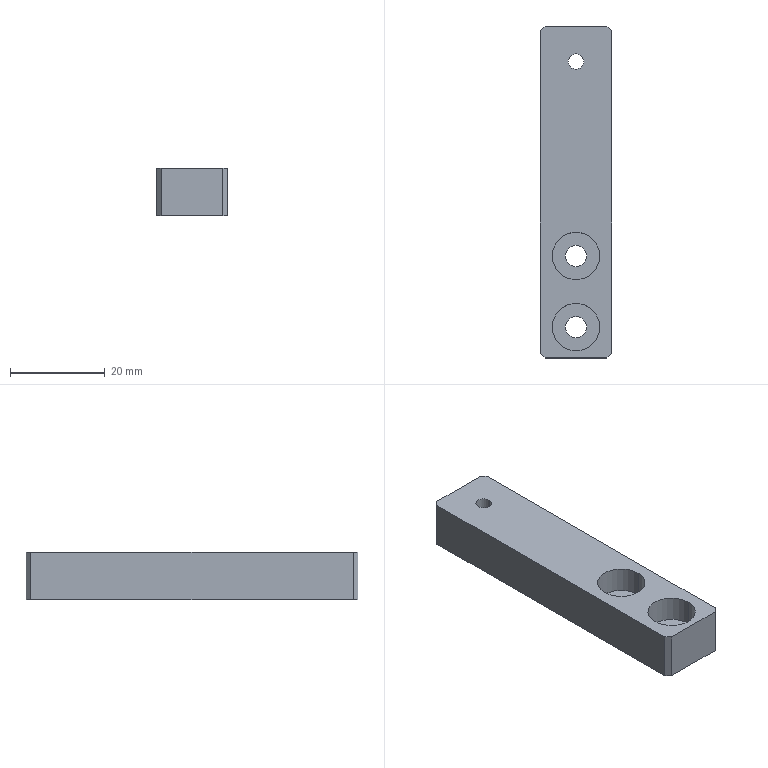Part | STEP file | 1 solid | 22 faces | box 15 x 70 x 10 mm | volume 9387 mm3 | plane 12 | cylinder 10 | commonest cylinder face diameters 4.5 x4 10 x4 3.3 x2